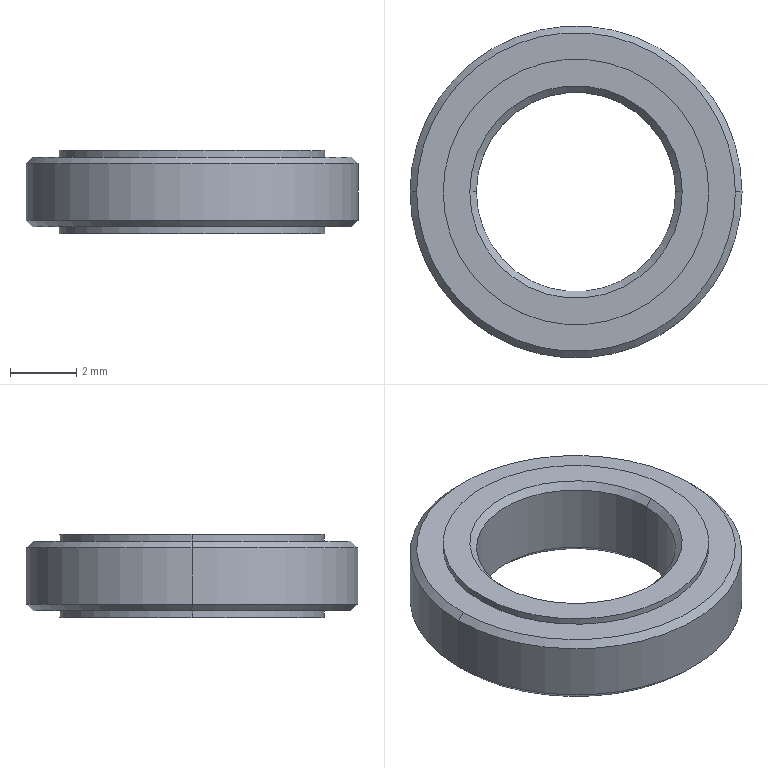Part | NX | features BREP 1 | 1 solid | 20 faces | box 10 x 10 x 2.5 mm | volume 112.343 mm3 | cone 8 | cylinder 8 | plane 4 | commonest cylinder face diameters 8 x4 6 x2 10 x2
STEP:
#1=CARTESIAN_POINT('',(4.8,0.,1.05));
#2=VERTEX_POINT('',#1);
#3=CARTESIAN_POINT('',(5.,0.,0.85));
#4=VERTEX_POINT('',#3);
#5=CARTESIAN_POINT('',(4.8,0.,1.05));
#6=DIRECTION('',(0.7071,0.,-0.7071));
#7=VECTOR('',#6,1000.);
#8=LINE('',#5,#7);
#9=EDGE_CURVE('',#2,#4,#8,.T.);
#10=ORIENTED_EDGE('',*,*,#9,.F.);
#11=CARTESIAN_POINT('',(-4.8,0.,1.05));
#12=VERTEX_POINT('',#11);
#13=CARTESIAN_POINT('',(0.,0.,1.05));
#14=DIRECTION('',(0.,0.,1.));
#15=DIRECTION('',(1.,0.,0.));
#16=AXIS2_PLACEMENT_3D('',#13,#14,#15);
#17=CIRCLE('',#16,4.8);
#18=EDGE_CURVE('',#12,#2,#17,.T.);
#19=ORIENTED_EDGE('',*,*,#18,.F.);
#20=CARTESIAN_POINT('',(-5.,0.,0.85));
#21=VERTEX_POINT('',#20);
#22=CARTESIAN_POINT('',(-4.8,0.,1.05));
#23=DIRECTION('',(-0.7071,0.,-0.7071));
#24=VECTOR('',#23,1000.);
#25=LINE('',#22,#24);
#26=EDGE_CURVE('',#12,#21,#25,.T.);
#27=ORIENTED_EDGE('',*,*,#26,.T.);
#28=CARTESIAN_POINT('',(0.,0.,0.85));
#29=DIRECTION('',(0.,0.,-1.));
#30=DIRECTION('',(1.,0.,0.));
#31=AXIS2_PLACEMENT_3D('',#28,#29,#30);
#32=CIRCLE('',#31,5.);
#33=EDGE_CURVE('',#4,#21,#32,.T.);
#34=ORIENTED_EDGE('',*,*,#33,.F.);
#35=EDGE_LOOP('',(#10,#19,#27,#34));
#36=FACE_BOUND('',#35,.T.);
#37=CARTESIAN_POINT('',(0.,0.,1.05));
#38=DIRECTION('',(0.,0.,-1.));
#39=DIRECTION('',(-1.,0.,0.));
#40=AXIS2_PLACEMENT_3D('',#37,#38,#39);
#41=CONICAL_SURFACE('',#40,4.8,0.7854);
#42=ADVANCED_FACE('',(#36),#41,.T.);
#43=CARTESIAN_POINT('',(-5.,0.,-0.85));
#44=VERTEX_POINT('',#43);
#45=CARTESIAN_POINT('',(-4.8,0.,-1.05));
#46=VERTEX_POINT('',#45);
#47=CARTESIAN_POINT('',(-5.,0.,-0.85));
#48=DIRECTION('',(-0.7071,0.,0.7071));
#49=VECTOR('',#48,1000.);
#50=LINE('',#47,#49);
#51=EDGE_CURVE('',#44,#46,#50,.F.);
#52=ORIENTED_EDGE('',*,*,#51,.T.);
#53=CARTESIAN_POINT('',(4.8,0.,-1.05));
#54=VERTEX_POINT('',#53);
#55=CARTESIAN_POINT('',(0.,0.,-1.05));
#56=DIRECTION('',(0.,0.,-1.));
#57=DIRECTION('',(-1.,0.,0.));
#58=AXIS2_PLACEMENT_3D('',#55,#56,#57);
#59=CIRCLE('',#58,4.8);
#60=EDGE_CURVE('',#54,#46,#59,.T.);
#61=ORIENTED_EDGE('',*,*,#60,.F.);
#62=CARTESIAN_POINT('',(5.,0.,-0.85));
#63=VERTEX_POINT('',#62);
#64=CARTESIAN_POINT('',(5.,0.,-0.85));
#65=DIRECTION('',(0.7071,0.,0.7071));
#66=VECTOR('',#65,1000.);
#67=LINE('',#64,#66);
#68=EDGE_CURVE('',#63,#54,#67,.F.);
#69=ORIENTED_EDGE('',*,*,#68,.F.);
#70=CARTESIAN_POINT('',(0.,0.,-0.85));
#71=DIRECTION('',(0.,0.,1.));
#72=DIRECTION('',(-1.,0.,0.));
#73=AXIS2_PLACEMENT_3D('',#70,#71,#72);
#74=CIRCLE('',#73,5.);
#75=EDGE_CURVE('',#44,#63,#74,.T.);
#76=ORIENTED_EDGE('',*,*,#75,.F.);
#77=EDGE_LOOP('',(#52,#61,#69,#76));
#78=FACE_BOUND('',#77,.T.);
#79=CARTESIAN_POINT('',(0.,0.,-0.85));
#80=DIRECTION('',(0.,0.,1.));
#81=DIRECTION('',(1.,0.,0.));
#82=AXIS2_PLACEMENT_3D('',#79,#80,#81);
#83=CONICAL_SURFACE('',#82,5.,0.7854);
#84=ADVANCED_FACE('',(#78),#83,.T.);
#85=CARTESIAN_POINT('',(-3.2,0.,1.25));
#86=VERTEX_POINT('',#85);
#87=CARTESIAN_POINT('',(-3.,0.,1.05));
#88=VERTEX_POINT('',#87);
#89=CARTESIAN_POINT('',(-3.,0.,1.05));
#90=DIRECTION('',(-0.7071,0.,0.7071));
#91=VECTOR('',#90,1000.);
#92=LINE('',#89,#91);
#93=EDGE_CURVE('',#86,#88,#92,.F.);
#94=ORIENTED_EDGE('',*,*,#93,.T.);
#95=CARTESIAN_POINT('',(3.,0.,1.05));
#96=VERTEX_POINT('',#95);
#97=CARTESIAN_POINT('',(0.,0.,1.05));
#98=DIRECTION('',(0.,0.,1.));
#99=DIRECTION('',(1.,0.,0.));
#100=AXIS2_PLACEMENT_3D('',#97,#98,#99);
#101=CIRCLE('',#100,3.);
#102=EDGE_CURVE('',#96,#88,#101,.T.);
#103=ORIENTED_EDGE('',*,*,#102,.F.);
#104=CARTESIAN_POINT('',(3.2,0.,1.25));
#105=VERTEX_POINT('',#104);
#106=CARTESIAN_POINT('',(3.,0.,1.05));
#107=DIRECTION('',(0.7071,0.,0.7071));
#108=VECTOR('',#107,1000.);
#109=LINE('',#106,#108);
#110=EDGE_CURVE('',#105,#96,#109,.F.);
#111=ORIENTED_EDGE('',*,*,#110,.F.);
#112=CARTESIAN_POINT('',(0.,0.,1.25));
#113=DIRECTION('',(0.,0.,-1.));
#114=DIRECTION('',(1.,0.,0.));
#115=AXIS2_PLACEMENT_3D('',#112,#113,#114);
#116=CIRCLE('',#115,3.2);
#117=EDGE_CURVE('',#86,#105,#116,.T.);
#118=ORIENTED_EDGE('',*,*,#117,.F.);
#119=EDGE_LOOP('',(#94,#103,#111,#118));
#120=FACE_BOUND('',#119,.T.);
#121=CARTESIAN_POINT('',(0.,0.,1.05));
#122=DIRECTION('',(0.,0.,1.));
#123=DIRECTION('',(1.,0.,0.));
#124=AXIS2_PLACEMENT_3D('',#121,#122,#123);
#125=CONICAL_SURFACE('',#124,3.,0.7854);
#126=ADVANCED_FACE('',(#120),#125,.F.);
#127=CARTESIAN_POINT('',(3.,0.,-1.05));
#128=VERTEX_POINT('',#127);
#129=CARTESIAN_POINT('',(3.2,0.,-1.25));
#130=VERTEX_POINT('',#129);
#131=CARTESIAN_POINT('',(3.2,0.,-1.25));
#132=DIRECTION('',(0.7071,0.,-0.7071));
#133=VECTOR('',#132,1000.);
#134=LINE('',#131,#133);
#135=EDGE_CURVE('',#128,#130,#134,.T.);
#136=ORIENTED_EDGE('',*,*,#135,.F.);
#137=CARTESIAN_POINT('',(-3.,0.,-1.05));
#138=VERTEX_POINT('',#137);
#139=CARTESIAN_POINT('',(0.,0.,-1.05));
#140=DIRECTION('',(0.,0.,-1.));
#141=DIRECTION('',(1.,0.,0.));
#142=AXIS2_PLACEMENT_3D('',#139,#140,#141);
#143=CIRCLE('',#142,3.);
#144=EDGE_CURVE('',#138,#128,#143,.T.);
#145=ORIENTED_EDGE('',*,*,#144,.F.);
#146=CARTESIAN_POINT('',(-3.2,0.,-1.25));
#147=VERTEX_POINT('',#146);
#148=CARTESIAN_POINT('',(-3.2,0.,-1.25));
#149=DIRECTION('',(-0.7071,0.,-0.7071));
#150=VECTOR('',#149,1000.);
#151=LINE('',#148,#150);
#152=EDGE_CURVE('',#138,#147,#151,.T.);
#153=ORIENTED_EDGE('',*,*,#152,.T.);
#154=CARTESIAN_POINT('',(0.,0.,-1.25));
#155=DIRECTION('',(0.,0.,1.));
#156=DIRECTION('',(1.,0.,0.));
#157=AXIS2_PLACEMENT_3D('',#154,#155,#156);
#158=CIRCLE('',#157,3.2);
#159=EDGE_CURVE('',#130,#147,#158,.T.);
#160=ORIENTED_EDGE('',*,*,#159,.F.);
#161=EDGE_LOOP('',(#136,#145,#153,#160));
#162=FACE_BOUND('',#161,.T.);
#163=CARTESIAN_POINT('',(0.,0.,-1.25));
#164=DIRECTION('',(0.,0.,-1.));
#165=DIRECTION('',(-1.,0.,0.));
#166=AXIS2_PLACEMENT_3D('',#163,#164,#165);
#167=CONICAL_SURFACE('',#166,3.2,0.7854);
#168=ADVANCED_FACE('',(#162),#167,.F.);
#169=CARTESIAN_POINT('',(4.,0.,-1.05));
#170=VERTEX_POINT('',#169);
#171=CARTESIAN_POINT('',(-4.,0.,-1.05));
#172=VERTEX_POINT('',#171);
#173=CARTESIAN_POINT('',(0.,0.,-1.05));
#174=DIRECTION('',(0.,0.,1.));
#175=DIRECTION('',(1.,0.,0.));
#176=AXIS2_PLACEMENT_3D('',#173,#174,#175);
#177=CIRCLE('',#176,4.);
#178=EDGE_CURVE('',#170,#172,#177,.T.);
#179=ORIENTED_EDGE('',*,*,#178,.T.);
#180=CARTESIAN_POINT('',(0.,0.,-1.05));
#181=DIRECTION('',(0.,0.,1.));
#182=DIRECTION('',(1.,0.,0.));
#183=AXIS2_PLACEMENT_3D('',#180,#181,#182);
#184=CIRCLE('',#183,4.);
#185=EDGE_CURVE('',#172,#170,#184,.T.);
#186=ORIENTED_EDGE('',*,*,#185,.T.);
#187=EDGE_LOOP('',(#179,#186));
#188=FACE_BOUND('',#187,.T.);
#189=ORIENTED_EDGE('',*,*,#60,.T.);
#190=CARTESIAN_POINT('',(0.,0.,-1.05));
#191=DIRECTION('',(0.,0.,-1.));
#192=DIRECTION('',(-1.,0.,0.));
#193=AXIS2_PLACEMENT_3D('',#190,#191,#192);
#194=CIRCLE('',#193,4.8);
#195=EDGE_CURVE('',#46,#54,#194,.T.);
#196=ORIENTED_EDGE('',*,*,#195,.T.);
#197=EDGE_LOOP('',(#189,#196));
#198=FACE_BOUND('',#197,.T.);
#199=CARTESIAN_POINT('',(0.,5.,-1.05));
#200=DIRECTION('',(0.,0.,-1.));
#201=DIRECTION('',(-1.,0.,0.));
#202=AXIS2_PLACEMENT_3D('',#199,#200,#201);
#203=PLANE('',#202);
#204=ADVANCED_FACE('',(#188,#198),#203,.T.);
#205=CARTESIAN_POINT('',(-4.,0.,-1.25));
#206=VERTEX_POINT('',#205);
#207=CARTESIAN_POINT('',(-4.,0.,0.));
#208=DIRECTION('',(0.,0.,1.));
#209=VECTOR('',#208,1000.);
#210=LINE('',#207,#209);
#211=EDGE_CURVE('',#172,#206,#210,.F.);
#212=ORIENTED_EDGE('',*,*,#211,.T.);
#213=CARTESIAN_POINT('',(4.,0.,-1.25));
#214=VERTEX_POINT('',#213);
#215=CARTESIAN_POINT('',(0.,0.,-1.25));
#216=DIRECTION('',(0.,0.,1.));
#217=DIRECTION('',(1.,0.,0.));
#218=AXIS2_PLACEMENT_3D('',#215,#216,#217);
#219=CIRCLE('',#218,4.);
#220=EDGE_CURVE('',#206,#214,#219,.T.);
#221=ORIENTED_EDGE('',*,*,#220,.T.);
#222=CARTESIAN_POINT('',(4.,0.,0.));
#223=DIRECTION('',(0.,0.,1.));
#224=VECTOR('',#223,1000.);
#225=LINE('',#222,#224);
#226=EDGE_CURVE('',#170,#214,#225,.F.);
#227=ORIENTED_EDGE('',*,*,#226,.F.);
#228=ORIENTED_EDGE('',*,*,#185,.F.);
#229=EDGE_LOOP('',(#212,#221,#227,#228));
#230=FACE_BOUND('',#229,.T.);
#231=CARTESIAN_POINT('',(0.,0.,0.));
#232=DIRECTION('',(0.,0.,1.));
#233=DIRECTION('',(1.,0.,0.));
#234=AXIS2_PLACEMENT_3D('',#231,#232,#233);
#235=CYLINDRICAL_SURFACE('',#234,4.);
#236=ADVANCED_FACE('',(#230),#235,.T.);
#237=CARTESIAN_POINT('',(4.,0.,1.05));
#238=VERTEX_POINT('',#237);
#239=CARTESIAN_POINT('',(-4.,0.,1.05));
#240=VERTEX_POINT('',#239);
#241=CARTESIAN_POINT('',(0.,0.,1.05));
#242=DIRECTION('',(0.,0.,1.));
#243=DIRECTION('',(1.,0.,0.));
#244=AXIS2_PLACEMENT_3D('',#241,#242,#243);
#245=CIRCLE('',#244,4.);
#246=EDGE_CURVE('',#238,#240,#245,.T.);
#247=ORIENTED_EDGE('',*,*,#246,.F.);
#248=CARTESIAN_POINT('',(0.,0.,1.05));
#249=DIRECTION('',(0.,0.,1.));
#250=DIRECTION('',(1.,0.,0.));
#251=AXIS2_PLACEMENT_3D('',#248,#249,#250);
#252=CIRCLE('',#251,4.);
#253=EDGE_CURVE('',#240,#238,#252,.T.);
#254=ORIENTED_EDGE('',*,*,#253,.F.);
#255=EDGE_LOOP('',(#247,#254));
#256=FACE_BOUND('',#255,.T.);
#257=ORIENTED_EDGE('',*,*,#18,.T.);
#258=CARTESIAN_POINT('',(0.,0.,1.05));
#259=DIRECTION('',(0.,0.,1.));
#260=DIRECTION('',(1.,0.,0.));
#261=AXIS2_PLACEMENT_3D('',#258,#259,#260);
#262=CIRCLE('',#261,4.8);
#263=EDGE_CURVE('',#2,#12,#262,.T.);
#264=ORIENTED_EDGE('',*,*,#263,.T.);
#265=EDGE_LOOP('',(#257,#264));
#266=FACE_BOUND('',#265,.T.);
#267=CARTESIAN_POINT('',(0.,5.,1.05));
#268=DIRECTION('',(0.,0.,1.));
#269=DIRECTION('',(1.,0.,0.));
#270=AXIS2_PLACEMENT_3D('',#267,#268,#269);
#271=PLANE('',#270);
#272=ADVANCED_FACE('',(#256,#266),#271,.T.);
#273=CARTESIAN_POINT('',(-4.,0.,1.25));
#274=VERTEX_POINT('',#273);
#275=CARTESIAN_POINT('',(-4.,0.,0.));
#276=DIRECTION('',(0.,0.,1.));
#277=VECTOR('',#276,1000.);
#278=LINE('',#275,#277);
#279=EDGE_CURVE('',#274,#240,#278,.F.);
#280=ORIENTED_EDGE('',*,*,#279,.T.);
#281=ORIENTED_EDGE('',*,*,#253,.T.);
#282=CARTESIAN_POINT('',(4.,0.,1.25));
#283=VERTEX_POINT('',#282);
#284=CARTESIAN_POINT('',(4.,0.,0.));
#285=DIRECTION('',(0.,0.,1.));
#286=VECTOR('',#285,1000.);
#287=LINE('',#284,#286);
#288=EDGE_CURVE('',#283,#238,#287,.F.);
#289=ORIENTED_EDGE('',*,*,#288,.F.);
#290=CARTESIAN_POINT('',(0.,0.,1.25));
#291=DIRECTION('',(0.,0.,1.));
#292=DIRECTION('',(1.,0.,0.));
#293=AXIS2_PLACEMENT_3D('',#290,#291,#292);
#294=CIRCLE('',#293,4.);
#295=EDGE_CURVE('',#274,#283,#294,.T.);
#296=ORIENTED_EDGE('',*,*,#295,.F.);
#297=EDGE_LOOP('',(#280,#281,#289,#296));
#298=FACE_BOUND('',#297,.T.);
#299=CARTESIAN_POINT('',(0.,0.,0.));
#300=DIRECTION('',(0.,0.,1.));
#301=DIRECTION('',(1.,0.,0.));
#302=AXIS2_PLACEMENT_3D('',#299,#300,#301);
#303=CYLINDRICAL_SURFACE('',#302,4.);
#304=ADVANCED_FACE('',(#298),#303,.T.);
#305=CARTESIAN_POINT('',(3.,0.,1.25));
#306=DIRECTION('',(0.,0.,-1.));
#307=VECTOR('',#306,1000.);
#308=LINE('',#305,#307);
#309=EDGE_CURVE('',#96,#128,#308,.T.);
#310=ORIENTED_EDGE('',*,*,#309,.F.);
#311=ORIENTED_EDGE('',*,*,#102,.T.);
#312=CARTESIAN_POINT('',(-3.,0.,1.25));
#313=DIRECTION('',(0.,0.,-1.));
#314=VECTOR('',#313,1000.);
#315=LINE('',#312,#314);
#316=EDGE_CURVE('',#88,#138,#315,.T.);
#317=ORIENTED_EDGE('',*,*,#316,.T.);
#318=ORIENTED_EDGE('',*,*,#144,.T.);
#319=EDGE_LOOP('',(#310,#311,#317,#318));
#320=FACE_BOUND('',#319,.T.);
#321=CARTESIAN_POINT('',(0.,0.,1.25));
#322=DIRECTION('',(0.,0.,-1.));
#323=DIRECTION('',(-1.,0.,0.));
#324=AXIS2_PLACEMENT_3D('',#321,#322,#323);
#325=CYLINDRICAL_SURFACE('',#324,3.);
#326=ADVANCED_FACE('',(#320),#325,.F.);
#327=CARTESIAN_POINT('',(0.,0.,1.25));
#328=DIRECTION('',(0.,0.,1.));
#329=DIRECTION('',(1.,0.,0.));
#330=AXIS2_PLACEMENT_3D('',#327,#328,#329);
#331=CIRCLE('',#330,4.);
#332=EDGE_CURVE('',#283,#274,#331,.T.);
#333=ORIENTED_EDGE('',*,*,#332,.T.);
#334=ORIENTED_EDGE('',*,*,#295,.T.);
#335=EDGE_LOOP('',(#333,#334));
#336=FACE_BOUND('',#335,.T.);
#337=CARTESIAN_POINT('',(0.,0.,1.25));
#338=DIRECTION('',(0.,0.,-1.));
#339=DIRECTION('',(1.,0.,0.));
#340=AXIS2_PLACEMENT_3D('',#337,#338,#339);
#341=CIRCLE('',#340,3.2);
#342=EDGE_CURVE('',#105,#86,#341,.T.);
#343=ORIENTED_EDGE('',*,*,#342,.T.);
#344=ORIENTED_EDGE('',*,*,#117,.T.);
#345=EDGE_LOOP('',(#343,#344));
#346=FACE_BOUND('',#345,.T.);
#347=CARTESIAN_POINT('',(0.,0.,1.25));
#348=DIRECTION('',(0.,0.,1.));
#349=DIRECTION('',(1.,0.,0.));
#350=AXIS2_PLACEMENT_3D('',#347,#348,#349);
#351=PLANE('',#350);
#352=ADVANCED_FACE('',(#336,#346),#351,.T.);
#353=CARTESIAN_POINT('',(0.,0.,-1.25));
#354=DIRECTION('',(0.,0.,1.));
#355=DIRECTION('',(1.,0.,0.));
#356=AXIS2_PLACEMENT_3D('',#353,#354,#355);
#357=CIRCLE('',#356,4.);
#358=EDGE_CURVE('',#214,#206,#357,.T.);
#359=ORIENTED_EDGE('',*,*,#358,.F.);
#360=ORIENTED_EDGE('',*,*,#220,.F.);
#361=EDGE_LOOP('',(#359,#360));
#362=FACE_BOUND('',#361,.T.);
#363=CARTESIAN_POINT('',(0.,0.,-1.25));
#364=DIRECTION('',(0.,0.,1.));
#365=DIRECTION('',(1.,0.,0.));
#366=AXIS2_PLACEMENT_3D('',#363,#364,#365);
#367=CIRCLE('',#366,3.2);
#368=EDGE_CURVE('',#147,#130,#367,.T.);
#369=ORIENTED_EDGE('',*,*,#368,.T.);
#370=ORIENTED_EDGE('',*,*,#159,.T.);
#371=EDGE_LOOP('',(#369,#370));
#372=FACE_BOUND('',#371,.T.);
#373=CARTESIAN_POINT('',(0.,0.,-1.25));
#374=DIRECTION('',(0.,0.,1.));
#375=DIRECTION('',(1.,0.,0.));
#376=AXIS2_PLACEMENT_3D('',#373,#374,#375);
#377=PLANE('',#376);
#378=ADVANCED_FACE('',(#362,#372),#377,.F.);
#379=CARTESIAN_POINT('',(5.,0.,1.25));
#380=DIRECTION('',(0.,0.,-1.));
#381=VECTOR('',#380,1000.);
#382=LINE('',#379,#381);
#383=EDGE_CURVE('',#4,#63,#382,.T.);
#384=ORIENTED_EDGE('',*,*,#383,.F.);
#385=ORIENTED_EDGE('',*,*,#33,.T.);
#386=CARTESIAN_POINT('',(-5.,0.,1.25));
#387=DIRECTION('',(0.,0.,-1.));
#388=VECTOR('',#387,1000.);
#389=LINE('',#386,#388);
#390=EDGE_CURVE('',#21,#44,#389,.T.);
#391=ORIENTED_EDGE('',*,*,#390,.T.);
#392=ORIENTED_EDGE('',*,*,#75,.T.);
#393=EDGE_LOOP('',(#384,#385,#391,#392));
#394=FACE_BOUND('',#393,.T.);
#395=CARTESIAN_POINT('',(0.,0.,1.25));
#396=DIRECTION('',(0.,0.,-1.));
#397=DIRECTION('',(-1.,0.,0.));
#398=AXIS2_PLACEMENT_3D('',#395,#396,#397);
#399=CYLINDRICAL_SURFACE('',#398,5.);
#400=ADVANCED_FACE('',(#394),#399,.T.);
#401=CARTESIAN_POINT('',(0.,0.,0.85));
#402=DIRECTION('',(0.,0.,-1.));
#403=DIRECTION('',(1.,0.,0.));
#404=AXIS2_PLACEMENT_3D('',#401,#402,#403);
#405=CIRCLE('',#404,5.);
#406=EDGE_CURVE('',#21,#4,#405,.T.);
#407=ORIENTED_EDGE('',*,*,#406,.T.);
#408=ORIENTED_EDGE('',*,*,#383,.T.);
#409=CARTESIAN_POINT('',(0.,0.,-0.85));
#410=DIRECTION('',(0.,0.,1.));
#411=DIRECTION('',(-1.,0.,0.));
#412=AXIS2_PLACEMENT_3D('',#409,#410,#411);
#413=CIRCLE('',#412,5.);
#414=EDGE_CURVE('',#63,#44,#413,.T.);
#415=ORIENTED_EDGE('',*,*,#414,.T.);
#416=ORIENTED_EDGE('',*,*,#390,.F.);
#417=EDGE_LOOP('',(#407,#408,#415,#416));
#418=FACE_BOUND('',#417,.T.);
#419=CARTESIAN_POINT('',(0.,0.,1.25));
#420=DIRECTION('',(0.,0.,-1.));
#421=DIRECTION('',(-1.,0.,0.));
#422=AXIS2_PLACEMENT_3D('',#419,#420,#421);
#423=CYLINDRICAL_SURFACE('',#422,5.);
#424=ADVANCED_FACE('',(#418),#423,.T.);
#425=CARTESIAN_POINT('',(0.,0.,1.05));
#426=DIRECTION('',(0.,0.,1.));
#427=DIRECTION('',(1.,0.,0.));
#428=AXIS2_PLACEMENT_3D('',#425,#426,#427);
#429=CIRCLE('',#428,3.);
#430=EDGE_CURVE('',#88,#96,#429,.T.);
#431=ORIENTED_EDGE('',*,*,#430,.T.);
#432=ORIENTED_EDGE('',*,*,#309,.T.);
#433=CARTESIAN_POINT('',(0.,0.,-1.05));
#434=DIRECTION('',(0.,0.,-1.));
#435=DIRECTION('',(1.,0.,0.));
#436=AXIS2_PLACEMENT_3D('',#433,#434,#435);
#437=CIRCLE('',#436,3.);
#438=EDGE_CURVE('',#128,#138,#437,.T.);
#439=ORIENTED_EDGE('',*,*,#438,.T.);
#440=ORIENTED_EDGE('',*,*,#316,.F.);
#441=EDGE_LOOP('',(#431,#432,#439,#440));
#442=FACE_BOUND('',#441,.T.);
#443=CARTESIAN_POINT('',(0.,0.,1.25));
#444=DIRECTION('',(0.,0.,-1.));
#445=DIRECTION('',(-1.,0.,0.));
#446=AXIS2_PLACEMENT_3D('',#443,#444,#445);
#447=CYLINDRICAL_SURFACE('',#446,3.);
#448=ADVANCED_FACE('',(#442),#447,.F.);
#449=ORIENTED_EDGE('',*,*,#246,.T.);
#450=ORIENTED_EDGE('',*,*,#279,.F.);
#451=ORIENTED_EDGE('',*,*,#332,.F.);
#452=ORIENTED_EDGE('',*,*,#288,.T.);
#453=EDGE_LOOP('',(#449,#450,#451,#452));
#454=FACE_BOUND('',#453,.T.);
#455=CARTESIAN_POINT('',(0.,0.,0.));
#456=DIRECTION('',(0.,0.,1.));
#457=DIRECTION('',(1.,0.,0.));
#458=AXIS2_PLACEMENT_3D('',#455,#456,#457);
#459=CYLINDRICAL_SURFACE('',#458,4.);
#460=ADVANCED_FACE('',(#454),#459,.T.);
#461=ORIENTED_EDGE('',*,*,#358,.T.);
#462=ORIENTED_EDGE('',*,*,#211,.F.);
#463=ORIENTED_EDGE('',*,*,#178,.F.);
#464=ORIENTED_EDGE('',*,*,#226,.T.);
#465=EDGE_LOOP('',(#461,#462,#463,#464));
#466=FACE_BOUND('',#465,.T.);
#467=CARTESIAN_POINT('',(0.,0.,0.));
#468=DIRECTION('',(0.,0.,1.));
#469=DIRECTION('',(1.,0.,0.));
#470=AXIS2_PLACEMENT_3D('',#467,#468,#469);
#471=CYLINDRICAL_SURFACE('',#470,4.);
#472=ADVANCED_FACE('',(#466),#471,.T.);
#473=ORIENTED_EDGE('',*,*,#438,.F.);
#474=ORIENTED_EDGE('',*,*,#135,.T.);
#475=ORIENTED_EDGE('',*,*,#368,.F.);
#476=ORIENTED_EDGE('',*,*,#152,.F.);
#477=EDGE_LOOP('',(#473,#474,#475,#476));
#478=FACE_BOUND('',#477,.T.);
#479=CARTESIAN_POINT('',(0.,0.,-1.25));
#480=DIRECTION('',(0.,0.,-1.));
#481=DIRECTION('',(-1.,0.,0.));
#482=AXIS2_PLACEMENT_3D('',#479,#480,#481);
#483=CONICAL_SURFACE('',#482,3.2,0.7854);
#484=ADVANCED_FACE('',(#478),#483,.F.);
#485=ORIENTED_EDGE('',*,*,#430,.F.);
#486=ORIENTED_EDGE('',*,*,#93,.F.);
#487=ORIENTED_EDGE('',*,*,#342,.F.);
#488=ORIENTED_EDGE('',*,*,#110,.T.);
#489=EDGE_LOOP('',(#485,#486,#487,#488));
#490=FACE_BOUND('',#489,.T.);
#491=CARTESIAN_POINT('',(0.,0.,1.05));
#492=DIRECTION('',(0.,0.,1.));
#493=DIRECTION('',(1.,0.,0.));
#494=AXIS2_PLACEMENT_3D('',#491,#492,#493);
#495=CONICAL_SURFACE('',#494,3.,0.7854);
#496=ADVANCED_FACE('',(#490),#495,.F.);
#497=ORIENTED_EDGE('',*,*,#195,.F.);
#498=ORIENTED_EDGE('',*,*,#51,.F.);
#499=ORIENTED_EDGE('',*,*,#414,.F.);
#500=ORIENTED_EDGE('',*,*,#68,.T.);
#501=EDGE_LOOP('',(#497,#498,#499,#500));
#502=FACE_BOUND('',#501,.T.);
#503=CARTESIAN_POINT('',(0.,0.,-0.85));
#504=DIRECTION('',(0.,0.,1.));
#505=DIRECTION('',(1.,0.,0.));
#506=AXIS2_PLACEMENT_3D('',#503,#504,#505);
#507=CONICAL_SURFACE('',#506,5.,0.7854);
#508=ADVANCED_FACE('',(#502),#507,.T.);
#509=ORIENTED_EDGE('',*,*,#263,.F.);
#510=ORIENTED_EDGE('',*,*,#9,.T.);
#511=ORIENTED_EDGE('',*,*,#406,.F.);
#512=ORIENTED_EDGE('',*,*,#26,.F.);
#513=EDGE_LOOP('',(#509,#510,#511,#512));
#514=FACE_BOUND('',#513,.T.);
#515=CARTESIAN_POINT('',(0.,0.,1.05));
#516=DIRECTION('',(0.,0.,-1.));
#517=DIRECTION('',(-1.,0.,0.));
#518=AXIS2_PLACEMENT_3D('',#515,#516,#517);
#519=CONICAL_SURFACE('',#518,4.8,0.7854);
#520=ADVANCED_FACE('',(#514),#519,.T.);
#521=CLOSED_SHELL('',(#42,#84,#126,#168,#204,#236,#272,#304,#326,#352,#378,#400,#424,#448,#460,#472,#484,#496,#508,#520));
#522=MANIFOLD_SOLID_BREP('',#521);
#523=(LENGTH_UNIT()NAMED_UNIT(*)SI_UNIT(.MILLI.,.METRE.));
#524=UNCERTAINTY_MEASURE_WITH_UNIT(LENGTH_MEASURE(0.00001),#523,'','');
#525=(NAMED_UNIT(*)PLANE_ANGLE_UNIT()SI_UNIT($,.RADIAN.));
#526=(NAMED_UNIT(*)SI_UNIT($,.STERADIAN.)SOLID_ANGLE_UNIT());
#527=(GEOMETRIC_REPRESENTATION_CONTEXT(3)GLOBAL_UNCERTAINTY_ASSIGNED_CONTEXT((#524))GLOBAL_UNIT_ASSIGNED_CONTEXT((#523,#525,#526))REPRESENTATION_CONTEXT('',''));
#528=ADVANCED_BREP_SHAPE_REPRESENTATION('',(#522),#527);